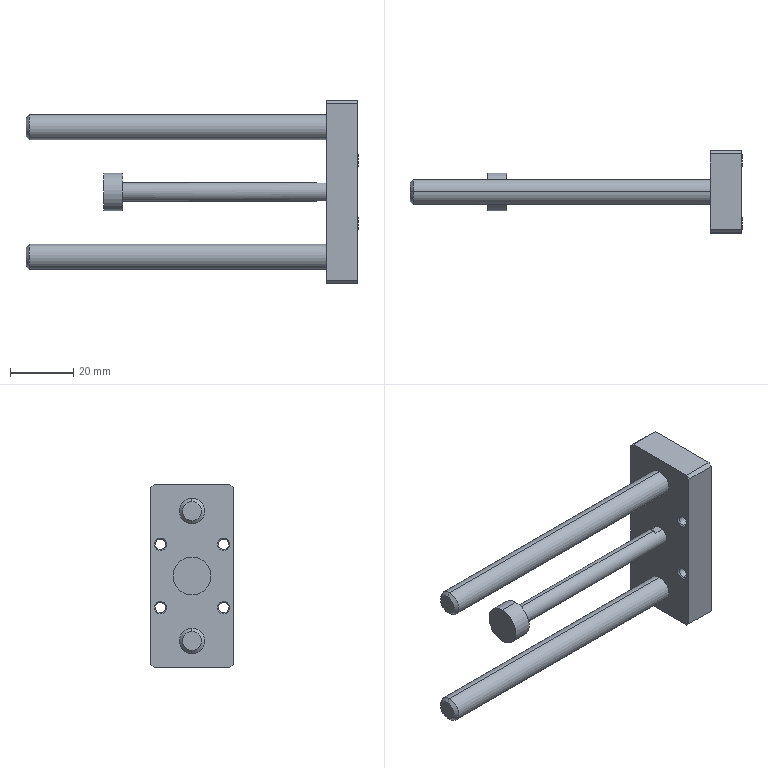Part | SolidWorks | features BaseBody 1 | 1 solid | 144 faces | box 105 x 26 x 58 mm | volume 26314 mm3 | cylinder 83 | cone 28 | plane 27 | spline 6 | commonest cylinder face diameters 1.378 x21 0.788 x16 3.242 x12 8 x12 0.787 x8 7 x6